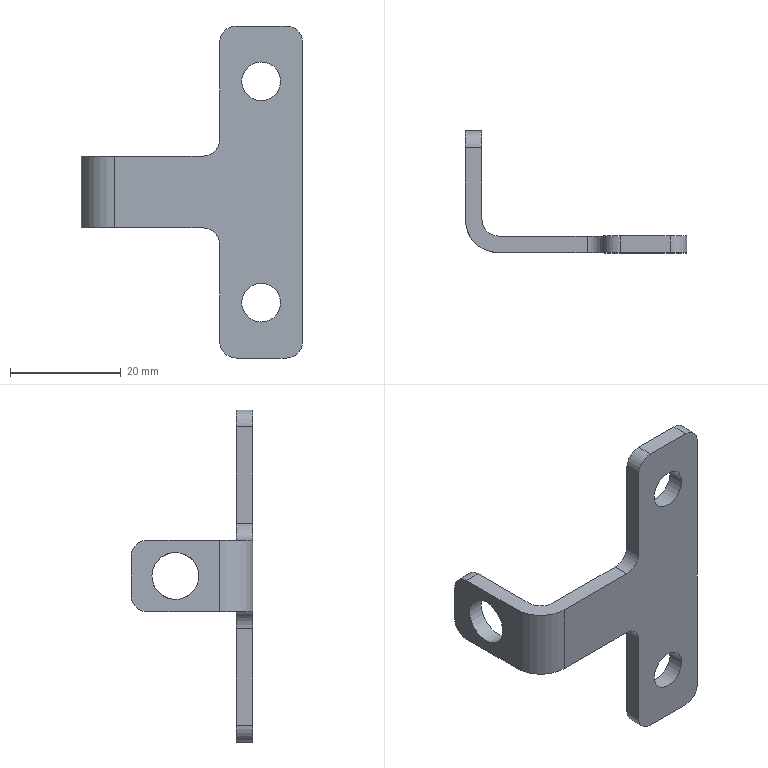Part | NX | features BREP 1 | 1 solid | 25 faces | box 40 x 22 x 60 mm | volume 3916 mm3 | cylinder 13 | plane 12 | commonest cylinder face diameters 6 x9 7 x2 8.5 x1 12 x1
STEP:
#1=CARTESIAN_POINT('',(28.,0.,-30.));
#2=VERTEX_POINT('',#1);
#3=CARTESIAN_POINT('',(37.,0.,-30.));
#4=VERTEX_POINT('',#3);
#5=CARTESIAN_POINT('',(0.,0.,-30.));
#6=DIRECTION('',(1.,0.,0.));
#7=VECTOR('',#6,1000.);
#8=LINE('',#5,#7);
#9=EDGE_CURVE('',#2,#4,#8,.T.);
#10=ORIENTED_EDGE('',*,*,#9,.F.);
#11=CARTESIAN_POINT('',(28.,3.,-30.));
#12=VERTEX_POINT('',#11);
#13=CARTESIAN_POINT('',(28.,3.,-30.));
#14=DIRECTION('',(0.,1.,0.));
#15=VECTOR('',#14,1000.);
#16=LINE('',#13,#15);
#17=EDGE_CURVE('',#2,#12,#16,.T.);
#18=ORIENTED_EDGE('',*,*,#17,.T.);
#19=CARTESIAN_POINT('',(37.,3.,-30.));
#20=VERTEX_POINT('',#19);
#21=CARTESIAN_POINT('',(0.,3.,-30.));
#22=DIRECTION('',(1.,0.,0.));
#23=VECTOR('',#22,1000.);
#24=LINE('',#21,#23);
#25=EDGE_CURVE('',#12,#20,#24,.T.);
#26=ORIENTED_EDGE('',*,*,#25,.T.);
#27=CARTESIAN_POINT('',(37.,6.,-30.));
#28=DIRECTION('',(0.,-1.,0.));
#29=VECTOR('',#28,1000.);
#30=LINE('',#27,#29);
#31=EDGE_CURVE('',#20,#4,#30,.T.);
#32=ORIENTED_EDGE('',*,*,#31,.T.);
#33=EDGE_LOOP('',(#10,#18,#26,#32));
#34=FACE_BOUND('',#33,.T.);
#35=CARTESIAN_POINT('',(3.,6.,-30.));
#36=DIRECTION('',(0.,0.,-1.));
#37=DIRECTION('',(1.,0.,0.));
#38=AXIS2_PLACEMENT_3D('',#35,#36,#37);
#39=PLANE('',#38);
#40=ADVANCED_FACE('',(#34),#39,.T.);
#41=CARTESIAN_POINT('',(32.5,0.,23.5));
#42=VERTEX_POINT('',#41);
#43=CARTESIAN_POINT('',(32.5,0.,20.));
#44=DIRECTION('',(0.,1.,0.));
#45=DIRECTION('',(0.,0.,1.));
#46=AXIS2_PLACEMENT_3D('',#43,#44,#45);
#47=CIRCLE('',#46,3.5);
#48=EDGE_CURVE('',#42,#42,#47,.T.);
#49=ORIENTED_EDGE('',*,*,#48,.T.);
#50=EDGE_LOOP('',(#49));
#51=FACE_BOUND('',#50,.T.);
#52=CARTESIAN_POINT('',(32.5,0.,-16.5));
#53=VERTEX_POINT('',#52);
#54=CARTESIAN_POINT('',(32.5,0.,-20.));
#55=DIRECTION('',(0.,1.,0.));
#56=DIRECTION('',(0.,0.,1.));
#57=AXIS2_PLACEMENT_3D('',#54,#55,#56);
#58=CIRCLE('',#57,3.5);
#59=EDGE_CURVE('',#53,#53,#58,.T.);
#60=ORIENTED_EDGE('',*,*,#59,.T.);
#61=EDGE_LOOP('',(#60));
#62=FACE_BOUND('',#61,.T.);
#63=CARTESIAN_POINT('',(25.,0.,-27.));
#64=VERTEX_POINT('',#63);
#65=CARTESIAN_POINT('',(25.,0.,-9.5));
#66=VERTEX_POINT('',#65);
#67=CARTESIAN_POINT('',(25.,0.,-6.5));
#68=DIRECTION('',(0.,0.,1.));
#69=VECTOR('',#68,1000.);
#70=LINE('',#67,#69);
#71=EDGE_CURVE('',#64,#66,#70,.T.);
#72=ORIENTED_EDGE('',*,*,#71,.F.);
#73=CARTESIAN_POINT('',(28.,0.,-27.));
#74=DIRECTION('',(0.,-1.,0.));
#75=DIRECTION('',(0.,0.,1.));
#76=AXIS2_PLACEMENT_3D('',#73,#74,#75);
#77=CIRCLE('',#76,3.);
#78=EDGE_CURVE('',#64,#2,#77,.T.);
#79=ORIENTED_EDGE('',*,*,#78,.T.);
#80=ORIENTED_EDGE('',*,*,#9,.T.);
#81=CARTESIAN_POINT('',(40.,0.,-27.));
#82=VERTEX_POINT('',#81);
#83=CARTESIAN_POINT('',(37.,0.,-27.));
#84=DIRECTION('',(0.,-1.,0.));
#85=DIRECTION('',(0.,0.,1.));
#86=AXIS2_PLACEMENT_3D('',#83,#84,#85);
#87=CIRCLE('',#86,3.);
#88=EDGE_CURVE('',#4,#82,#87,.T.);
#89=ORIENTED_EDGE('',*,*,#88,.T.);
#90=CARTESIAN_POINT('',(40.,0.,27.));
#91=VERTEX_POINT('',#90);
#92=CARTESIAN_POINT('',(40.,0.,30.));
#93=DIRECTION('',(0.,0.,-1.));
#94=VECTOR('',#93,1000.);
#95=LINE('',#92,#94);
#96=EDGE_CURVE('',#91,#82,#95,.T.);
#97=ORIENTED_EDGE('',*,*,#96,.F.);
#98=CARTESIAN_POINT('',(37.,0.,30.));
#99=VERTEX_POINT('',#98);
#100=CARTESIAN_POINT('',(37.,0.,27.));
#101=DIRECTION('',(0.,-1.,0.));
#102=DIRECTION('',(0.,0.,1.));
#103=AXIS2_PLACEMENT_3D('',#100,#101,#102);
#104=CIRCLE('',#103,3.);
#105=EDGE_CURVE('',#91,#99,#104,.T.);
#106=ORIENTED_EDGE('',*,*,#105,.T.);
#107=CARTESIAN_POINT('',(28.,0.,30.));
#108=VERTEX_POINT('',#107);
#109=CARTESIAN_POINT('',(0.,0.,30.));
#110=DIRECTION('',(1.,0.,0.));
#111=VECTOR('',#110,1000.);
#112=LINE('',#109,#111);
#113=EDGE_CURVE('',#108,#99,#112,.T.);
#114=ORIENTED_EDGE('',*,*,#113,.F.);
#115=CARTESIAN_POINT('',(25.,0.,27.));
#116=VERTEX_POINT('',#115);
#117=CARTESIAN_POINT('',(28.,0.,27.));
#118=DIRECTION('',(0.,-1.,0.));
#119=DIRECTION('',(0.,0.,1.));
#120=AXIS2_PLACEMENT_3D('',#117,#118,#119);
#121=CIRCLE('',#120,3.);
#122=EDGE_CURVE('',#108,#116,#121,.T.);
#123=ORIENTED_EDGE('',*,*,#122,.T.);
#124=CARTESIAN_POINT('',(25.,0.,9.5));
#125=VERTEX_POINT('',#124);
#126=CARTESIAN_POINT('',(25.,0.,30.));
#127=DIRECTION('',(0.,0.,1.));
#128=VECTOR('',#127,1000.);
#129=LINE('',#126,#128);
#130=EDGE_CURVE('',#125,#116,#129,.T.);
#131=ORIENTED_EDGE('',*,*,#130,.F.);
#132=CARTESIAN_POINT('',(22.,0.,6.5));
#133=VERTEX_POINT('',#132);
#134=CARTESIAN_POINT('',(22.,0.,9.5));
#135=DIRECTION('',(0.,1.,0.));
#136=DIRECTION('',(0.,0.,1.));
#137=AXIS2_PLACEMENT_3D('',#134,#135,#136);
#138=CIRCLE('',#137,3.);
#139=EDGE_CURVE('',#125,#133,#138,.T.);
#140=ORIENTED_EDGE('',*,*,#139,.T.);
#141=CARTESIAN_POINT('',(6.,0.,6.5));
#142=VERTEX_POINT('',#141);
#143=CARTESIAN_POINT('',(25.,0.,6.5));
#144=DIRECTION('',(1.,0.,0.));
#145=VECTOR('',#144,1000.);
#146=LINE('',#143,#145);
#147=EDGE_CURVE('',#142,#133,#146,.T.);
#148=ORIENTED_EDGE('',*,*,#147,.F.);
#149=CARTESIAN_POINT('',(6.,0.,-6.5));
#150=VERTEX_POINT('',#149);
#151=CARTESIAN_POINT('',(6.,0.,30.));
#152=DIRECTION('',(0.,0.,-1.));
#153=VECTOR('',#152,1000.);
#154=LINE('',#151,#153);
#155=EDGE_CURVE('',#142,#150,#154,.T.);
#156=ORIENTED_EDGE('',*,*,#155,.T.);
#157=CARTESIAN_POINT('',(22.,0.,-6.5));
#158=VERTEX_POINT('',#157);
#159=CARTESIAN_POINT('',(0.,0.,-6.5));
#160=DIRECTION('',(-1.,0.,0.));
#161=VECTOR('',#160,1000.);
#162=LINE('',#159,#161);
#163=EDGE_CURVE('',#158,#150,#162,.T.);
#164=ORIENTED_EDGE('',*,*,#163,.F.);
#165=CARTESIAN_POINT('',(22.,0.,-9.5));
#166=DIRECTION('',(0.,1.,0.));
#167=DIRECTION('',(0.,0.,1.));
#168=AXIS2_PLACEMENT_3D('',#165,#166,#167);
#169=CIRCLE('',#168,3.);
#170=EDGE_CURVE('',#158,#66,#169,.T.);
#171=ORIENTED_EDGE('',*,*,#170,.T.);
#172=EDGE_LOOP('',(#72,#79,#80,#89,#97,#106,#114,#123,#131,#140,#148,#156,#164,#171));
#173=FACE_BOUND('',#172,.T.);
#174=CARTESIAN_POINT('',(0.,0.,30.));
#175=DIRECTION('',(0.,1.,0.));
#176=DIRECTION('',(0.,0.,-1.));
#177=AXIS2_PLACEMENT_3D('',#174,#175,#176);
#178=PLANE('',#177);
#179=ADVANCED_FACE('',(#51,#62,#173),#178,.F.);
#180=ORIENTED_EDGE('',*,*,#96,.T.);
#181=CARTESIAN_POINT('',(40.,3.,-27.));
#182=VERTEX_POINT('',#181);
#183=CARTESIAN_POINT('',(40.,3.,-27.));
#184=DIRECTION('',(0.,1.,0.));
#185=VECTOR('',#184,1000.);
#186=LINE('',#183,#185);
#187=EDGE_CURVE('',#82,#182,#186,.T.);
#188=ORIENTED_EDGE('',*,*,#187,.T.);
#189=CARTESIAN_POINT('',(40.,3.,27.));
#190=VERTEX_POINT('',#189);
#191=CARTESIAN_POINT('',(40.,3.,30.));
#192=DIRECTION('',(0.,0.,-1.));
#193=VECTOR('',#192,1000.);
#194=LINE('',#191,#193);
#195=EDGE_CURVE('',#190,#182,#194,.T.);
#196=ORIENTED_EDGE('',*,*,#195,.F.);
#197=CARTESIAN_POINT('',(40.,3.,27.));
#198=DIRECTION('',(0.,-1.,0.));
#199=VECTOR('',#198,1000.);
#200=LINE('',#197,#199);
#201=EDGE_CURVE('',#190,#91,#200,.T.);
#202=ORIENTED_EDGE('',*,*,#201,.T.);
#203=EDGE_LOOP('',(#180,#188,#196,#202));
#204=FACE_BOUND('',#203,.T.);
#205=CARTESIAN_POINT('',(40.,3.,30.));
#206=DIRECTION('',(1.,0.,0.));
#207=DIRECTION('',(0.,0.,1.));
#208=AXIS2_PLACEMENT_3D('',#205,#206,#207);
#209=PLANE('',#208);
#210=ADVANCED_FACE('',(#204),#209,.T.);
#211=CARTESIAN_POINT('',(32.5,3.,23.5));
#212=VERTEX_POINT('',#211);
#213=CARTESIAN_POINT('',(32.5,3.,20.));
#214=DIRECTION('',(0.,1.,0.));
#215=DIRECTION('',(0.,0.,1.));
#216=AXIS2_PLACEMENT_3D('',#213,#214,#215);
#217=CIRCLE('',#216,3.5);
#218=EDGE_CURVE('',#212,#212,#217,.T.);
#219=ORIENTED_EDGE('',*,*,#218,.F.);
#220=EDGE_LOOP('',(#219));
#221=FACE_BOUND('',#220,.T.);
#222=CARTESIAN_POINT('',(32.5,3.,-16.5));
#223=VERTEX_POINT('',#222);
#224=CARTESIAN_POINT('',(32.5,3.,-20.));
#225=DIRECTION('',(0.,1.,0.));
#226=DIRECTION('',(0.,0.,1.));
#227=AXIS2_PLACEMENT_3D('',#224,#225,#226);
#228=CIRCLE('',#227,3.5);
#229=EDGE_CURVE('',#223,#223,#228,.T.);
#230=ORIENTED_EDGE('',*,*,#229,.F.);
#231=EDGE_LOOP('',(#230));
#232=FACE_BOUND('',#231,.T.);
#233=ORIENTED_EDGE('',*,*,#25,.F.);
#234=CARTESIAN_POINT('',(25.,3.,-27.));
#235=VERTEX_POINT('',#234);
#236=CARTESIAN_POINT('',(28.,3.,-27.));
#237=DIRECTION('',(0.,1.,0.));
#238=DIRECTION('',(0.,0.,1.));
#239=AXIS2_PLACEMENT_3D('',#236,#237,#238);
#240=CIRCLE('',#239,3.);
#241=EDGE_CURVE('',#12,#235,#240,.T.);
#242=ORIENTED_EDGE('',*,*,#241,.T.);
#243=CARTESIAN_POINT('',(25.,3.,-9.5));
#244=VERTEX_POINT('',#243);
#245=CARTESIAN_POINT('',(25.,3.,30.));
#246=DIRECTION('',(0.,0.,-1.));
#247=VECTOR('',#246,1000.);
#248=LINE('',#245,#247);
#249=EDGE_CURVE('',#244,#235,#248,.T.);
#250=ORIENTED_EDGE('',*,*,#249,.F.);
#251=CARTESIAN_POINT('',(22.,3.,-6.5));
#252=VERTEX_POINT('',#251);
#253=CARTESIAN_POINT('',(22.,3.,-9.5));
#254=DIRECTION('',(0.,-1.,0.));
#255=DIRECTION('',(0.,0.,1.));
#256=AXIS2_PLACEMENT_3D('',#253,#254,#255);
#257=CIRCLE('',#256,3.);
#258=EDGE_CURVE('',#244,#252,#257,.T.);
#259=ORIENTED_EDGE('',*,*,#258,.T.);
#260=CARTESIAN_POINT('',(6.,3.,-6.5));
#261=VERTEX_POINT('',#260);
#262=CARTESIAN_POINT('',(0.,3.,-6.5));
#263=DIRECTION('',(1.,0.,0.));
#264=VECTOR('',#263,1000.);
#265=LINE('',#262,#264);
#266=EDGE_CURVE('',#261,#252,#265,.T.);
#267=ORIENTED_EDGE('',*,*,#266,.F.);
#268=CARTESIAN_POINT('',(6.,3.,6.5));
#269=VERTEX_POINT('',#268);
#270=CARTESIAN_POINT('',(6.,3.,30.));
#271=DIRECTION('',(0.,0.,-1.));
#272=VECTOR('',#271,1000.);
#273=LINE('',#270,#272);
#274=EDGE_CURVE('',#269,#261,#273,.T.);
#275=ORIENTED_EDGE('',*,*,#274,.F.);
#276=CARTESIAN_POINT('',(22.,3.,6.5));
#277=VERTEX_POINT('',#276);
#278=CARTESIAN_POINT('',(0.,3.,6.5));
#279=DIRECTION('',(-1.,0.,0.));
#280=VECTOR('',#279,1000.);
#281=LINE('',#278,#280);
#282=EDGE_CURVE('',#277,#269,#281,.T.);
#283=ORIENTED_EDGE('',*,*,#282,.F.);
#284=CARTESIAN_POINT('',(25.,3.,9.5));
#285=VERTEX_POINT('',#284);
#286=CARTESIAN_POINT('',(22.,3.,9.5));
#287=DIRECTION('',(0.,-1.,0.));
#288=DIRECTION('',(0.,0.,1.));
#289=AXIS2_PLACEMENT_3D('',#286,#287,#288);
#290=CIRCLE('',#289,3.);
#291=EDGE_CURVE('',#277,#285,#290,.T.);
#292=ORIENTED_EDGE('',*,*,#291,.T.);
#293=CARTESIAN_POINT('',(25.,3.,27.));
#294=VERTEX_POINT('',#293);
#295=CARTESIAN_POINT('',(25.,3.,30.));
#296=DIRECTION('',(0.,0.,-1.));
#297=VECTOR('',#296,1000.);
#298=LINE('',#295,#297);
#299=EDGE_CURVE('',#294,#285,#298,.T.);
#300=ORIENTED_EDGE('',*,*,#299,.F.);
#301=CARTESIAN_POINT('',(28.,3.,30.));
#302=VERTEX_POINT('',#301);
#303=CARTESIAN_POINT('',(28.,3.,27.));
#304=DIRECTION('',(0.,1.,0.));
#305=DIRECTION('',(0.,0.,1.));
#306=AXIS2_PLACEMENT_3D('',#303,#304,#305);
#307=CIRCLE('',#306,3.);
#308=EDGE_CURVE('',#294,#302,#307,.T.);
#309=ORIENTED_EDGE('',*,*,#308,.T.);
#310=CARTESIAN_POINT('',(37.,3.,30.));
#311=VERTEX_POINT('',#310);
#312=CARTESIAN_POINT('',(0.,3.,30.));
#313=DIRECTION('',(1.,0.,0.));
#314=VECTOR('',#313,1000.);
#315=LINE('',#312,#314);
#316=EDGE_CURVE('',#302,#311,#315,.T.);
#317=ORIENTED_EDGE('',*,*,#316,.T.);
#318=CARTESIAN_POINT('',(37.,3.,27.));
#319=DIRECTION('',(0.,1.,0.));
#320=DIRECTION('',(0.,0.,1.));
#321=AXIS2_PLACEMENT_3D('',#318,#319,#320);
#322=CIRCLE('',#321,3.);
#323=EDGE_CURVE('',#311,#190,#322,.T.);
#324=ORIENTED_EDGE('',*,*,#323,.T.);
#325=ORIENTED_EDGE('',*,*,#195,.T.);
#326=CARTESIAN_POINT('',(37.,3.,-27.));
#327=DIRECTION('',(0.,1.,0.));
#328=DIRECTION('',(0.,0.,1.));
#329=AXIS2_PLACEMENT_3D('',#326,#327,#328);
#330=CIRCLE('',#329,3.);
#331=EDGE_CURVE('',#182,#20,#330,.T.);
#332=ORIENTED_EDGE('',*,*,#331,.T.);
#333=EDGE_LOOP('',(#233,#242,#250,#259,#267,#275,#283,#292,#300,#309,#317,#324,#325,#332));
#334=FACE_BOUND('',#333,.T.);
#335=CARTESIAN_POINT('',(0.,3.,30.));
#336=DIRECTION('',(0.,1.,0.));
#337=DIRECTION('',(0.,0.,-1.));
#338=AXIS2_PLACEMENT_3D('',#335,#336,#337);
#339=PLANE('',#338);
#340=ADVANCED_FACE('',(#221,#232,#334),#339,.T.);
#341=CARTESIAN_POINT('',(3.,6.,6.5));
#342=VERTEX_POINT('',#341);
#343=CARTESIAN_POINT('',(6.,6.,6.5));
#344=DIRECTION('',(0.,0.,-1.));
#345=DIRECTION('',(-1.,0.,0.));
#346=AXIS2_PLACEMENT_3D('',#343,#344,#345);
#347=CIRCLE('',#346,3.);
#348=EDGE_CURVE('',#269,#342,#347,.T.);
#349=ORIENTED_EDGE('',*,*,#348,.F.);
#350=ORIENTED_EDGE('',*,*,#274,.T.);
#351=CARTESIAN_POINT('',(3.,6.,-6.5));
#352=VERTEX_POINT('',#351);
#353=CARTESIAN_POINT('',(6.,6.,-6.5));
#354=DIRECTION('',(0.,0.,1.));
#355=DIRECTION('',(1.,0.,0.));
#356=AXIS2_PLACEMENT_3D('',#353,#354,#355);
#357=CIRCLE('',#356,3.);
#358=EDGE_CURVE('',#352,#261,#357,.T.);
#359=ORIENTED_EDGE('',*,*,#358,.F.);
#360=CARTESIAN_POINT('',(3.,6.,30.));
#361=DIRECTION('',(0.,0.,-1.));
#362=VECTOR('',#361,1000.);
#363=LINE('',#360,#362);
#364=EDGE_CURVE('',#342,#352,#363,.T.);
#365=ORIENTED_EDGE('',*,*,#364,.F.);
#366=EDGE_LOOP('',(#349,#350,#359,#365));
#367=FACE_BOUND('',#366,.T.);
#368=CARTESIAN_POINT('',(6.,6.,30.));
#369=DIRECTION('',(0.,0.,-1.));
#370=DIRECTION('',(1.,0.,0.));
#371=AXIS2_PLACEMENT_3D('',#368,#369,#370);
#372=CYLINDRICAL_SURFACE('',#371,3.);
#373=ADVANCED_FACE('',(#367),#372,.F.);
#374=CARTESIAN_POINT('',(3.,18.25,0.));
#375=VERTEX_POINT('',#374);
#376=CARTESIAN_POINT('',(3.,14.,0.));
#377=DIRECTION('',(1.,0.,0.));
#378=DIRECTION('',(0.,1.,0.));
#379=AXIS2_PLACEMENT_3D('',#376,#377,#378);
#380=CIRCLE('',#379,4.25);
#381=EDGE_CURVE('',#375,#375,#380,.T.);
#382=ORIENTED_EDGE('',*,*,#381,.F.);
#383=EDGE_LOOP('',(#382));
#384=FACE_BOUND('',#383,.T.);
#385=CARTESIAN_POINT('',(3.,19.,-6.5));
#386=VERTEX_POINT('',#385);
#387=CARTESIAN_POINT('',(3.,22.,-6.5));
#388=DIRECTION('',(0.,-1.,0.));
#389=VECTOR('',#388,1000.);
#390=LINE('',#387,#389);
#391=EDGE_CURVE('',#386,#352,#390,.T.);
#392=ORIENTED_EDGE('',*,*,#391,.F.);
#393=CARTESIAN_POINT('',(3.,22.,-3.5));
#394=VERTEX_POINT('',#393);
#395=CARTESIAN_POINT('',(3.,19.,-3.5));
#396=DIRECTION('',(1.,0.,0.));
#397=DIRECTION('',(0.,1.,0.));
#398=AXIS2_PLACEMENT_3D('',#395,#396,#397);
#399=CIRCLE('',#398,3.);
#400=EDGE_CURVE('',#386,#394,#399,.T.);
#401=ORIENTED_EDGE('',*,*,#400,.T.);
#402=CARTESIAN_POINT('',(3.,22.,3.5));
#403=VERTEX_POINT('',#402);
#404=CARTESIAN_POINT('',(3.,22.,30.));
#405=DIRECTION('',(0.,0.,-1.));
#406=VECTOR('',#405,1000.);
#407=LINE('',#404,#406);
#408=EDGE_CURVE('',#403,#394,#407,.T.);
#409=ORIENTED_EDGE('',*,*,#408,.F.);
#410=CARTESIAN_POINT('',(3.,19.,6.5));
#411=VERTEX_POINT('',#410);
#412=CARTESIAN_POINT('',(3.,19.,3.5));
#413=DIRECTION('',(1.,0.,0.));
#414=DIRECTION('',(0.,1.,0.));
#415=AXIS2_PLACEMENT_3D('',#412,#413,#414);
#416=CIRCLE('',#415,3.);
#417=EDGE_CURVE('',#403,#411,#416,.T.);
#418=ORIENTED_EDGE('',*,*,#417,.T.);
#419=CARTESIAN_POINT('',(3.,22.,6.5));
#420=DIRECTION('',(0.,1.,0.));
#421=VECTOR('',#420,1000.);
#422=LINE('',#419,#421);
#423=EDGE_CURVE('',#342,#411,#422,.T.);
#424=ORIENTED_EDGE('',*,*,#423,.F.);
#425=ORIENTED_EDGE('',*,*,#364,.T.);
#426=EDGE_LOOP('',(#392,#401,#409,#418,#424,#425));
#427=FACE_BOUND('',#426,.T.);
#428=CARTESIAN_POINT('',(3.,22.,30.));
#429=DIRECTION('',(1.,0.,0.));
#430=DIRECTION('',(0.,-1.,0.));
#431=AXIS2_PLACEMENT_3D('',#428,#429,#430);
#432=PLANE('',#431);
#433=ADVANCED_FACE('',(#384,#427),#432,.T.);
#434=ORIENTED_EDGE('',*,*,#408,.T.);
#435=CARTESIAN_POINT('',(0.,22.,-3.5));
#436=VERTEX_POINT('',#435);
#437=CARTESIAN_POINT('',(0.,22.,-3.5));
#438=DIRECTION('',(-1.,0.,0.));
#439=VECTOR('',#438,1000.);
#440=LINE('',#437,#439);
#441=EDGE_CURVE('',#394,#436,#440,.T.);
#442=ORIENTED_EDGE('',*,*,#441,.T.);
#443=CARTESIAN_POINT('',(0.,22.,3.5));
#444=VERTEX_POINT('',#443);
#445=CARTESIAN_POINT('',(0.,22.,30.));
#446=DIRECTION('',(0.,0.,-1.));
#447=VECTOR('',#446,1000.);
#448=LINE('',#445,#447);
#449=EDGE_CURVE('',#444,#436,#448,.T.);
#450=ORIENTED_EDGE('',*,*,#449,.F.);
#451=CARTESIAN_POINT('',(3.,22.,3.5));
#452=DIRECTION('',(1.,0.,0.));
#453=VECTOR('',#452,1000.);
#454=LINE('',#451,#453);
#455=EDGE_CURVE('',#444,#403,#454,.T.);
#456=ORIENTED_EDGE('',*,*,#455,.T.);
#457=EDGE_LOOP('',(#434,#442,#450,#456));
#458=FACE_BOUND('',#457,.T.);
#459=CARTESIAN_POINT('',(0.,22.,30.));
#460=DIRECTION('',(0.,1.,0.));
#461=DIRECTION('',(0.,0.,-1.));
#462=AXIS2_PLACEMENT_3D('',#459,#460,#461);
#463=PLANE('',#462);
#464=ADVANCED_FACE('',(#458),#463,.T.);
#465=CARTESIAN_POINT('',(0.,14.,4.25));
#466=VERTEX_POINT('',#465);
#467=CARTESIAN_POINT('',(0.,14.,0.));
#468=DIRECTION('',(-1.,0.,0.));
#469=DIRECTION('',(0.,0.,1.));
#470=AXIS2_PLACEMENT_3D('',#467,#468,#469);
#471=CIRCLE('',#470,4.25);
#472=EDGE_CURVE('',#466,#466,#471,.T.);
#473=ORIENTED_EDGE('',*,*,#472,.F.);
#474=EDGE_LOOP('',(#473));
#475=FACE_BOUND('',#474,.T.);
#476=ORIENTED_EDGE('',*,*,#449,.T.);
#477=CARTESIAN_POINT('',(0.,19.,-6.5));
#478=VERTEX_POINT('',#477);
#479=CARTESIAN_POINT('',(0.,19.,-3.5));
#480=DIRECTION('',(-1.,0.,0.));
#481=DIRECTION('',(0.,1.,0.));
#482=AXIS2_PLACEMENT_3D('',#479,#480,#481);
#483=CIRCLE('',#482,3.);
#484=EDGE_CURVE('',#436,#478,#483,.T.);
#485=ORIENTED_EDGE('',*,*,#484,.T.);
#486=CARTESIAN_POINT('',(0.,6.,-6.5));
#487=VERTEX_POINT('',#486);
#488=CARTESIAN_POINT('',(0.,56.311,-6.5));
#489=DIRECTION('',(0.,-1.,0.));
#490=VECTOR('',#489,1000.);
#491=LINE('',#488,#490);
#492=EDGE_CURVE('',#478,#487,#491,.T.);
#493=ORIENTED_EDGE('',*,*,#492,.T.);
#494=CARTESIAN_POINT('',(0.,6.,6.5));
#495=VERTEX_POINT('',#494);
#496=CARTESIAN_POINT('',(0.,6.,30.));
#497=DIRECTION('',(0.,0.,-1.));
#498=VECTOR('',#497,1000.);
#499=LINE('',#496,#498);
#500=EDGE_CURVE('',#495,#487,#499,.T.);
#501=ORIENTED_EDGE('',*,*,#500,.F.);
#502=CARTESIAN_POINT('',(0.,19.,6.5));
#503=VERTEX_POINT('',#502);
#504=CARTESIAN_POINT('',(0.,56.311,6.5));
#505=DIRECTION('',(0.,-1.,0.));
#506=VECTOR('',#505,1000.);
#507=LINE('',#504,#506);
#508=EDGE_CURVE('',#503,#495,#507,.T.);
#509=ORIENTED_EDGE('',*,*,#508,.F.);
#510=CARTESIAN_POINT('',(0.,19.,3.5));
#511=DIRECTION('',(-1.,0.,0.));
#512=DIRECTION('',(0.,1.,0.));
#513=AXIS2_PLACEMENT_3D('',#510,#511,#512);
#514=CIRCLE('',#513,3.);
#515=EDGE_CURVE('',#503,#444,#514,.T.);
#516=ORIENTED_EDGE('',*,*,#515,.T.);
#517=EDGE_LOOP('',(#476,#485,#493,#501,#509,#516));
#518=FACE_BOUND('',#517,.T.);
#519=CARTESIAN_POINT('',(0.,22.,30.));
#520=DIRECTION('',(1.,0.,0.));
#521=DIRECTION('',(0.,-1.,0.));
#522=AXIS2_PLACEMENT_3D('',#519,#520,#521);
#523=PLANE('',#522);
#524=ADVANCED_FACE('',(#475,#518),#523,.F.);
#525=ORIENTED_EDGE('',*,*,#155,.F.);
#526=CARTESIAN_POINT('',(6.,6.,6.5));
#527=DIRECTION('',(0.,0.,-1.));
#528=DIRECTION('',(-1.,0.,0.));
#529=AXIS2_PLACEMENT_3D('',#526,#527,#528);
#530=CIRCLE('',#529,6.);
#531=EDGE_CURVE('',#142,#495,#530,.T.);
#532=ORIENTED_EDGE('',*,*,#531,.T.);
#533=ORIENTED_EDGE('',*,*,#500,.T.);
#534=CARTESIAN_POINT('',(6.,6.,-6.5));
#535=DIRECTION('',(0.,0.,1.));
#536=DIRECTION('',(1.,0.,0.));
#537=AXIS2_PLACEMENT_3D('',#534,#535,#536);
#538=CIRCLE('',#537,6.);
#539=EDGE_CURVE('',#487,#150,#538,.T.);
#540=ORIENTED_EDGE('',*,*,#539,.T.);
#541=EDGE_LOOP('',(#525,#532,#533,#540));
#542=FACE_BOUND('',#541,.T.);
#543=CARTESIAN_POINT('',(6.,6.,30.));
#544=DIRECTION('',(0.,0.,-1.));
#545=DIRECTION('',(1.,0.,0.));
#546=AXIS2_PLACEMENT_3D('',#543,#544,#545);
#547=CYLINDRICAL_SURFACE('',#546,6.);
#548=ADVANCED_FACE('',(#542),#547,.T.);
#549=ORIENTED_EDGE('',*,*,#316,.F.);
#550=CARTESIAN_POINT('',(28.,0.,30.));
#551=DIRECTION('',(0.,-1.,0.));
#552=VECTOR('',#551,1000.);
#553=LINE('',#550,#552);
#554=EDGE_CURVE('',#302,#108,#553,.T.);
#555=ORIENTED_EDGE('',*,*,#554,.T.);
#556=ORIENTED_EDGE('',*,*,#113,.T.);
#557=CARTESIAN_POINT('',(37.,6.,30.));
#558=DIRECTION('',(0.,1.,0.));
#559=VECTOR('',#558,1000.);
#560=LINE('',#557,#559);
#561=EDGE_CURVE('',#99,#311,#560,.T.);
#562=ORIENTED_EDGE('',*,*,#561,.T.);
#563=EDGE_LOOP('',(#549,#555,#556,#562));
#564=FACE_BOUND('',#563,.T.);
#565=CARTESIAN_POINT('',(6.,6.,30.));
#566=DIRECTION('',(0.,0.,1.));
#567=DIRECTION('',(-1.,0.,0.));
#568=AXIS2_PLACEMENT_3D('',#565,#566,#567);
#569=PLANE('',#568);
#570=ADVANCED_FACE('',(#564),#569,.T.);
#571=ORIENTED_EDGE('',*,*,#423,.T.);
#572=CARTESIAN_POINT('',(0.,19.,6.5));
#573=DIRECTION('',(-1.,0.,0.));
#574=VECTOR('',#573,1000.);
#575=LINE('',#572,#574);
#576=EDGE_CURVE('',#411,#503,#575,.T.);
#577=ORIENTED_EDGE('',*,*,#576,.T.);
#578=ORIENTED_EDGE('',*,*,#508,.T.);
#579=ORIENTED_EDGE('',*,*,#531,.F.);
#580=ORIENTED_EDGE('',*,*,#147,.T.);
#581=CARTESIAN_POINT('',(22.,3.,6.5));
#582=DIRECTION('',(0.,1.,0.));
#583=VECTOR('',#582,1000.);
#584=LINE('',#581,#583);
#585=EDGE_CURVE('',#133,#277,#584,.T.);
#586=ORIENTED_EDGE('',*,*,#585,.T.);
#587=ORIENTED_EDGE('',*,*,#282,.T.);
#588=ORIENTED_EDGE('',*,*,#348,.T.);
#589=EDGE_LOOP('',(#571,#577,#578,#579,#580,#586,#587,#588));
#590=FACE_BOUND('',#589,.T.);
#591=CARTESIAN_POINT('',(25.,56.311,6.5));
#592=DIRECTION('',(0.,0.,-1.));
#593=DIRECTION('',(1.,0.,0.));
#594=AXIS2_PLACEMENT_3D('',#591,#592,#593);
#595=PLANE('',#594);
#596=ADVANCED_FACE('',(#590),#595,.F.);
#597=ORIENTED_EDGE('',*,*,#130,.T.);
#598=CARTESIAN_POINT('',(25.,3.,27.));
#599=DIRECTION('',(0.,1.,0.));
#600=VECTOR('',#599,1000.);
#601=LINE('',#598,#600);
#602=EDGE_CURVE('',#116,#294,#601,.T.);
#603=ORIENTED_EDGE('',*,*,#602,.T.);
#604=ORIENTED_EDGE('',*,*,#299,.T.);
#605=CARTESIAN_POINT('',(25.,0.,9.5));
#606=DIRECTION('',(0.,-1.,0.));
#607=VECTOR('',#606,1000.);
#608=LINE('',#605,#607);
#609=EDGE_CURVE('',#285,#125,#608,.T.);
#610=ORIENTED_EDGE('',*,*,#609,.T.);
#611=EDGE_LOOP('',(#597,#603,#604,#610));
#612=FACE_BOUND('',#611,.T.);
#613=CARTESIAN_POINT('',(25.,56.311,30.));
#614=DIRECTION('',(1.,0.,0.));
#615=DIRECTION('',(0.,0.,1.));
#616=AXIS2_PLACEMENT_3D('',#613,#614,#615);
#617=PLANE('',#616);
#618=ADVANCED_FACE('',(#612),#617,.F.);
#619=ORIENTED_EDGE('',*,*,#492,.F.);
#620=CARTESIAN_POINT('',(3.,19.,-6.5));
#621=DIRECTION('',(1.,0.,0.));
#622=VECTOR('',#621,1000.);
#623=LINE('',#620,#622);
#624=EDGE_CURVE('',#478,#386,#623,.T.);
#625=ORIENTED_EDGE('',*,*,#624,.T.);
#626=ORIENTED_EDGE('',*,*,#391,.T.);
#627=ORIENTED_EDGE('',*,*,#358,.T.);
#628=ORIENTED_EDGE('',*,*,#266,.T.);
#629=CARTESIAN_POINT('',(22.,0.,-6.5));
#630=DIRECTION('',(0.,-1.,0.));
#631=VECTOR('',#630,1000.);
#632=LINE('',#629,#631);
#633=EDGE_CURVE('',#252,#158,#632,.T.);
#634=ORIENTED_EDGE('',*,*,#633,.T.);
#635=ORIENTED_EDGE('',*,*,#163,.T.);
#636=ORIENTED_EDGE('',*,*,#539,.F.);
#637=EDGE_LOOP('',(#619,#625,#626,#627,#628,#634,#635,#636));
#638=FACE_BOUND('',#637,.T.);
#639=CARTESIAN_POINT('',(0.,56.311,-6.5));
#640=DIRECTION('',(0.,0.,1.));
#641=DIRECTION('',(-1.,0.,0.));
#642=AXIS2_PLACEMENT_3D('',#639,#640,#641);
#643=PLANE('',#642);
#644=ADVANCED_FACE('',(#638),#643,.F.);
#645=ORIENTED_EDGE('',*,*,#71,.T.);
#646=CARTESIAN_POINT('',(25.,3.,-9.5));
#647=DIRECTION('',(0.,1.,0.));
#648=VECTOR('',#647,1000.);
#649=LINE('',#646,#648);
#650=EDGE_CURVE('',#66,#244,#649,.T.);
#651=ORIENTED_EDGE('',*,*,#650,.T.);
#652=ORIENTED_EDGE('',*,*,#249,.T.);
#653=CARTESIAN_POINT('',(25.,0.,-27.));
#654=DIRECTION('',(0.,-1.,0.));
#655=VECTOR('',#654,1000.);
#656=LINE('',#653,#655);
#657=EDGE_CURVE('',#235,#64,#656,.T.);
#658=ORIENTED_EDGE('',*,*,#657,.T.);
#659=EDGE_LOOP('',(#645,#651,#652,#658));
#660=FACE_BOUND('',#659,.T.);
#661=CARTESIAN_POINT('',(25.,56.311,-6.5));
#662=DIRECTION('',(1.,0.,0.));
#663=DIRECTION('',(0.,0.,1.));
#664=AXIS2_PLACEMENT_3D('',#661,#662,#663);
#665=PLANE('',#664);
#666=ADVANCED_FACE('',(#660),#665,.F.);
#667=ORIENTED_EDGE('',*,*,#381,.T.);
#668=EDGE_LOOP('',(#667));
#669=FACE_BOUND('',#668,.T.);
#670=ORIENTED_EDGE('',*,*,#472,.T.);
#671=EDGE_LOOP('',(#670));
#672=FACE_BOUND('',#671,.T.);
#673=CARTESIAN_POINT('',(0.,14.,0.));
#674=DIRECTION('',(-1.,0.,0.));
#675=DIRECTION('',(0.,0.,-1.));
#676=AXIS2_PLACEMENT_3D('',#673,#674,#675);
#677=CYLINDRICAL_SURFACE('',#676,4.25);
#678=ADVANCED_FACE('',(#669,#672),#677,.F.);
#679=ORIENTED_EDGE('',*,*,#59,.F.);
#680=EDGE_LOOP('',(#679));
#681=FACE_BOUND('',#680,.T.);
#682=ORIENTED_EDGE('',*,*,#229,.T.);
#683=EDGE_LOOP('',(#682));
#684=FACE_BOUND('',#683,.T.);
#685=CARTESIAN_POINT('',(32.5,3.,-20.));
#686=DIRECTION('',(0.,1.,0.));
#687=DIRECTION('',(0.,0.,-1.));
#688=AXIS2_PLACEMENT_3D('',#685,#686,#687);
#689=CYLINDRICAL_SURFACE('',#688,3.5);
#690=ADVANCED_FACE('',(#681,#684),#689,.F.);
#691=ORIENTED_EDGE('',*,*,#48,.F.);
#692=EDGE_LOOP('',(#691));
#693=FACE_BOUND('',#692,.T.);
#694=ORIENTED_EDGE('',*,*,#218,.T.);
#695=EDGE_LOOP('',(#694));
#696=FACE_BOUND('',#695,.T.);
#697=CARTESIAN_POINT('',(32.5,3.,20.));
#698=DIRECTION('',(0.,1.,0.));
#699=DIRECTION('',(0.,0.,-1.));
#700=AXIS2_PLACEMENT_3D('',#697,#698,#699);
#701=CYLINDRICAL_SURFACE('',#700,3.5);
#702=ADVANCED_FACE('',(#693,#696),#701,.F.);
#703=ORIENTED_EDGE('',*,*,#400,.F.);
#704=ORIENTED_EDGE('',*,*,#624,.F.);
#705=ORIENTED_EDGE('',*,*,#484,.F.);
#706=ORIENTED_EDGE('',*,*,#441,.F.);
#707=EDGE_LOOP('',(#703,#704,#705,#706));
#708=FACE_BOUND('',#707,.T.);
#709=CARTESIAN_POINT('',(0.,19.,-3.5));
#710=DIRECTION('',(1.,0.,0.));
#711=DIRECTION('',(0.,0.,1.));
#712=AXIS2_PLACEMENT_3D('',#709,#710,#711);
#713=CYLINDRICAL_SURFACE('',#712,3.);
#714=ADVANCED_FACE('',(#708),#713,.T.);
#715=ORIENTED_EDGE('',*,*,#515,.F.);
#716=ORIENTED_EDGE('',*,*,#576,.F.);
#717=ORIENTED_EDGE('',*,*,#417,.F.);
#718=ORIENTED_EDGE('',*,*,#455,.F.);
#719=EDGE_LOOP('',(#715,#716,#717,#718));
#720=FACE_BOUND('',#719,.T.);
#721=CARTESIAN_POINT('',(0.,19.,3.5));
#722=DIRECTION('',(-1.,0.,0.));
#723=DIRECTION('',(0.,0.,-1.));
#724=AXIS2_PLACEMENT_3D('',#721,#722,#723);
#725=CYLINDRICAL_SURFACE('',#724,3.);
#726=ADVANCED_FACE('',(#720),#725,.T.);
#727=ORIENTED_EDGE('',*,*,#258,.F.);
#728=ORIENTED_EDGE('',*,*,#650,.F.);
#729=ORIENTED_EDGE('',*,*,#170,.F.);
#730=ORIENTED_EDGE('',*,*,#633,.F.);
#731=EDGE_LOOP('',(#727,#728,#729,#730));
#732=FACE_BOUND('',#731,.T.);
#733=CARTESIAN_POINT('',(22.,56.311,-9.5));
#734=DIRECTION('',(0.,1.,0.));
#735=DIRECTION('',(0.,0.,-1.));
#736=AXIS2_PLACEMENT_3D('',#733,#734,#735);
#737=CYLINDRICAL_SURFACE('',#736,3.);
#738=ADVANCED_FACE('',(#732),#737,.F.);
#739=ORIENTED_EDGE('',*,*,#241,.F.);
#740=ORIENTED_EDGE('',*,*,#17,.F.);
#741=ORIENTED_EDGE('',*,*,#78,.F.);
#742=ORIENTED_EDGE('',*,*,#657,.F.);
#743=EDGE_LOOP('',(#739,#740,#741,#742));
#744=FACE_BOUND('',#743,.T.);
#745=CARTESIAN_POINT('',(28.,56.311,-27.));
#746=DIRECTION('',(0.,1.,0.));
#747=DIRECTION('',(0.,0.,-1.));
#748=AXIS2_PLACEMENT_3D('',#745,#746,#747);
#749=CYLINDRICAL_SURFACE('',#748,3.);
#750=ADVANCED_FACE('',(#744),#749,.T.);
#751=ORIENTED_EDGE('',*,*,#331,.F.);
#752=ORIENTED_EDGE('',*,*,#187,.F.);
#753=ORIENTED_EDGE('',*,*,#88,.F.);
#754=ORIENTED_EDGE('',*,*,#31,.F.);
#755=EDGE_LOOP('',(#751,#752,#753,#754));
#756=FACE_BOUND('',#755,.T.);
#757=CARTESIAN_POINT('',(37.,6.,-27.));
#758=DIRECTION('',(0.,-1.,0.));
#759=DIRECTION('',(0.,0.,1.));
#760=AXIS2_PLACEMENT_3D('',#757,#758,#759);
#761=CYLINDRICAL_SURFACE('',#760,3.);
#762=ADVANCED_FACE('',(#756),#761,.T.);
#763=ORIENTED_EDGE('',*,*,#122,.F.);
#764=ORIENTED_EDGE('',*,*,#554,.F.);
#765=ORIENTED_EDGE('',*,*,#308,.F.);
#766=ORIENTED_EDGE('',*,*,#602,.F.);
#767=EDGE_LOOP('',(#763,#764,#765,#766));
#768=FACE_BOUND('',#767,.T.);
#769=CARTESIAN_POINT('',(28.,56.311,27.));
#770=DIRECTION('',(0.,-1.,0.));
#771=DIRECTION('',(0.,0.,1.));
#772=AXIS2_PLACEMENT_3D('',#769,#770,#771);
#773=CYLINDRICAL_SURFACE('',#772,3.);
#774=ADVANCED_FACE('',(#768),#773,.T.);
#775=ORIENTED_EDGE('',*,*,#291,.F.);
#776=ORIENTED_EDGE('',*,*,#585,.F.);
#777=ORIENTED_EDGE('',*,*,#139,.F.);
#778=ORIENTED_EDGE('',*,*,#609,.F.);
#779=EDGE_LOOP('',(#775,#776,#777,#778));
#780=FACE_BOUND('',#779,.T.);
#781=CARTESIAN_POINT('',(22.,56.311,9.5));
#782=DIRECTION('',(0.,1.,0.));
#783=DIRECTION('',(0.,0.,-1.));
#784=AXIS2_PLACEMENT_3D('',#781,#782,#783);
#785=CYLINDRICAL_SURFACE('',#784,3.);
#786=ADVANCED_FACE('',(#780),#785,.F.);
#787=ORIENTED_EDGE('',*,*,#323,.F.);
#788=ORIENTED_EDGE('',*,*,#561,.F.);
#789=ORIENTED_EDGE('',*,*,#105,.F.);
#790=ORIENTED_EDGE('',*,*,#201,.F.);
#791=EDGE_LOOP('',(#787,#788,#789,#790));
#792=FACE_BOUND('',#791,.T.);
#793=CARTESIAN_POINT('',(37.,3.,27.));
#794=DIRECTION('',(0.,-1.,0.));
#795=DIRECTION('',(0.,0.,1.));
#796=AXIS2_PLACEMENT_3D('',#793,#794,#795);
#797=CYLINDRICAL_SURFACE('',#796,3.);
#798=ADVANCED_FACE('',(#792),#797,.T.);
#799=CLOSED_SHELL('',(#40,#179,#210,#340,#373,#433,#464,#524,#548,#570,#596,#618,#644,#666,#678,#690,#702,#714,#726,#738,#750,#762,#774,#786,#798));
#800=MANIFOLD_SOLID_BREP('',#799);
#801=(LENGTH_UNIT()NAMED_UNIT(*)SI_UNIT(.MILLI.,.METRE.));
#802=UNCERTAINTY_MEASURE_WITH_UNIT(LENGTH_MEASURE(0.00001),#801,'','');
#803=(NAMED_UNIT(*)PLANE_ANGLE_UNIT()SI_UNIT($,.RADIAN.));
#804=(NAMED_UNIT(*)SI_UNIT($,.STERADIAN.)SOLID_ANGLE_UNIT());
#805=(GEOMETRIC_REPRESENTATION_CONTEXT(3)GLOBAL_UNCERTAINTY_ASSIGNED_CONTEXT((#802))GLOBAL_UNIT_ASSIGNED_CONTEXT((#801,#803,#804))REPRESENTATION_CONTEXT('',''));
#806=ADVANCED_BREP_SHAPE_REPRESENTATION('',(#800),#805);